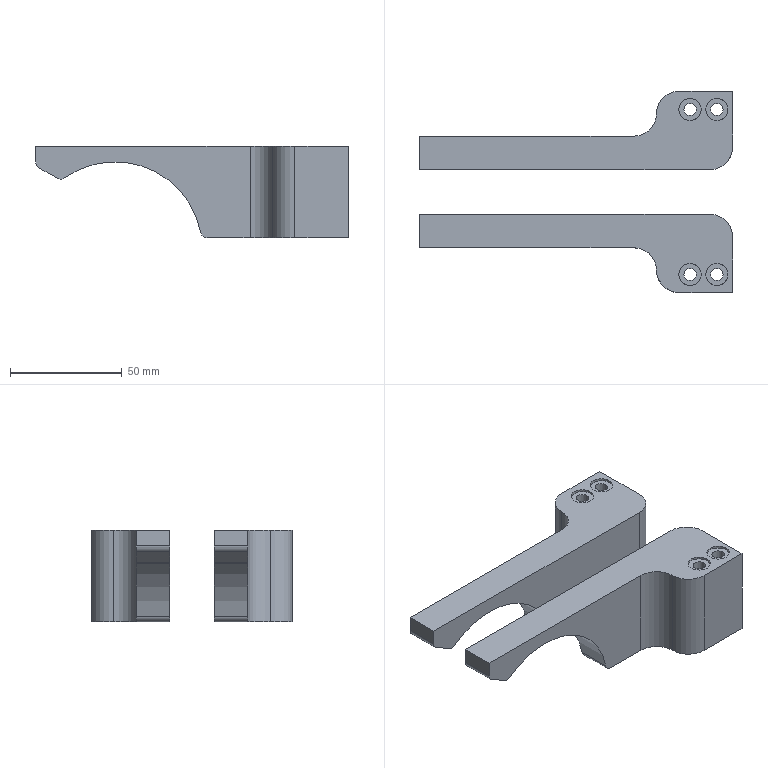NC program | NX | posted with a generic post | part box 140 x 90 x 41 mm
Lines 5312 to 6149 of 28919:
(FIXED_CONTOUR , TOOL : R4)
N10580 T08 M6
N10582 G54
N10584 G17 G0 G90 X6.198 Y-2.003 S9500 M3
N10586 G43 Z30. H8
N10588 Z4.4
N10590 G94 G1 Z0.371 F3000.
N10592 X6.29 Y-2.096 Z0.209
N10594 X6.41 Y-2.215 Z0.086
N10596 X6.548 Y-2.353 Z0.011
N10598 X6.695 Y-2.5 Z-0.011
N10600 X6.831 Y-2.637 Z-0.006
N10602 Y-2.773 Z-0.004
N10604 X6.558 Y-2.5 Z-0.014
N10606 X6.421 Z-0.017
N10608 X6.831 Y-2.91 Z-0.004
N10610 Y-3.046
N10612 X6.589 Y-2.804 Z-0.009
N10614 X6.427 Y-2.642 Z-0.015
N10616 X6.285 Y-2.5 Z-0.028
N10618 X6.148 Z-0.039
N10620 X6.427 Y-2.779 Z-0.013
N10622 X6.831 Y-3.183 Z-0.004
N10624 Y-3.318
N10626 X6.427 Y-2.914 Z-0.013
N10628 X6.145 Y-2.632 Z-0.037
N10630 X6.013 Y-2.5 Z-0.055
N10632 X5.877 Z-0.071
N10634 X6.181 Y-2.804 Z-0.032
N10636 X6.427 Y-3.05 Z-0.013
N10638 X6.831 Y-3.454 Z-0.004
N10640 Y-3.591
N10642 X6.427 Y-3.187 Z-0.013
N10644 X6.145 Y-2.905 Z-0.035
N10646 X5.863 Y-2.623 Z-0.07
N10648 X5.74 Y-2.5 Z-0.092
N10650 X5.605 Z-0.115
N10652 X5.863 Y-2.759 Z-0.068
N10654 X6.145 Y-3.041 Z-0.035
N10656 X6.427 Y-3.322 Z-0.013
N10658 X6.831 Y-3.726 Z-0.004
N10660 Y-3.86
N10662 X6.427 Y-3.456 Z-0.013
N10664 X6.145 Y-3.174 Z-0.035
N10666 X5.863 Y-2.892 Z-0.068
N10668 X5.582 Y-2.611 Z-0.117
N10670 X5.471 Y-2.5 Z-0.144
N10672 X5.336 Z-0.174
N10674 X5.582 Y-2.746 Z-0.115
N10676 X5.863 Y-3.027 Z-0.068
N10678 X6.145 Y-3.309 Z-0.035
N10680 X6.427 Y-3.591 Z-0.013
N10682 X6.831 Y-3.995 Z-0.004
N10684 Y-4.13
N10686 X6.427 Y-3.726 Z-0.013
N10688 X6.145 Y-3.445 Z-0.035
N10690 X5.863 Y-3.163 Z-0.068
N10692 X5.582 Y-2.881 Z-0.114
N10694 X5.201 Y-2.5 Z-0.206
N10696 X5.065 Z-0.238
N10698 X5.369 Y-2.804 Z-0.163
N10700 X5.582 Y-3.017 Z-0.114
N10702 X5.863 Y-3.298 Z-0.068
N10704 X6.145 Y-3.58 Z-0.035
N10706 X6.427 Y-3.862 Z-0.013
N10708 X6.831 Y-4.266 Z-0.004
N10710 Y-4.401
N10712 X6.427 Y-3.997 Z-0.013
N10714 X6.145 Y-3.715 Z-0.035
N10716 X5.863 Y-3.433 Z-0.068
N10718 X5.582 Y-3.152 Z-0.114
N10720 X5.234 Y-2.804 Z-0.194
N10722 X5.018 Y-2.588 Z-0.247
N10724 X4.93 Y-2.5 Z-0.273
N10726 X4.795 Z-0.309
N10728 X5.018 Y-2.723 Z-0.245
N10730 X5.3 Y-3.004 Z-0.178
N10732 X5.582 Y-3.286 Z-0.114
N10734 X5.863 Y-3.568 Z-0.068
N10736 X6.145 Y-3.85 Z-0.035
N10738 X6.427 Y-4.131 Z-0.013
N10740 X6.831 Y-4.536 Z-0.004
N10742 Y-4.667
N10744 X6.427 Y-4.263 Z-0.013
N10746 X6.145 Y-3.982 Z-0.035
N10748 X5.863 Y-3.7 Z-0.068
N10750 X5.582 Y-3.418 Z-0.114
N10752 X5.018 Y-2.855 Z-0.244
N10754 X4.736 Y-2.573 Z-0.324
N10756 X4.664 Y-2.5 Z-0.351
N10758 X4.531 Z-0.398
N10760 X4.736 Y-2.705 Z-0.322
N10762 X5.018 Y-2.987 Z-0.244
N10764 X5.582 Y-3.551 Z-0.114
N10766 X5.863 Y-3.832 Z-0.068
N10768 X6.145 Y-4.114 Z-0.035
N10770 X6.427 Y-4.396 Z-0.013
N10772 X6.831 Y-4.8 Z-0.004
N10774 Y-4.933
N10776 X6.427 Y-4.529 Z-0.013
N10778 X6.145 Y-4.247 Z-0.035
N10780 X5.863 Y-3.966 Z-0.068
N10782 X5.582 Y-3.684 Z-0.114
N10784 X5.018 Y-3.12 Z-0.244
N10786 X4.736 Y-2.839 Z-0.321
N10788 X4.455 Y-2.557 Z-0.424
N10790 X4.398 Y-2.5 Z-0.448
N10792 X4.265 Z-0.501
N10794 X4.455 Y-2.689 Z-0.422
N10796 X4.736 Y-2.971 Z-0.321
N10798 X5.018 Y-3.253 Z-0.244
N10800 X5.582 Y-3.816 Z-0.114
N10802 X5.863 Y-4.098 Z-0.068
N10804 X6.145 Y-4.38 Z-0.035
N10806 X6.427 Y-4.662 Z-0.013
N10808 X6.831 Y-5.066 Z-0.004
N10810 Y-5.198
N10812 X6.427 Y-4.794 Z-0.013
N10814 X6.145 Y-4.512 Z-0.035
N10816 X5.863 Y-4.23 Z-0.068
N10818 X5.582 Y-3.949 Z-0.114
N10820 X5.018 Y-3.385 Z-0.244
N10822 X4.736 Y-3.103 Z-0.321
N10824 X4.437 Y-2.804 Z-0.427
N10826 X4.133 Y-2.5 Z-0.555
N10828 X4.002 Z-0.608
N10830 X4.306 Y-2.804 Z-0.48
N10832 X4.455 Y-2.953 Z-0.42
N10834 X4.736 Y-3.234 Z-0.321
N10836 X5.018 Y-3.516 Z-0.244
N10838 X5.582 Y-4.08 Z-0.114
N10840 X5.863 Y-4.361 Z-0.068
N10842 X6.145 Y-4.643 Z-0.035
N10844 X6.427 Y-4.925 Z-0.013
N10846 X6.831 Y-5.329 Z-0.004
N10848 Y-5.459
N10850 X6.427 Y-5.055 Z-0.013
N10852 X6.145 Y-4.773 Z-0.035
N10854 X5.863 Y-4.491 Z-0.068
N10856 X5.582 Y-4.209 Z-0.114
N10858 X5.018 Y-3.646 Z-0.244
N10860 X4.736 Y-3.364 Z-0.321
N10862 X4.455 Y-3.082 Z-0.42
N10864 X4.176 Y-2.804 Z-0.532
N10866 X3.891 Y-2.519 Z-0.654
N10868 X3.872 Y-2.5 Z-0.663
N10870 X3.744 Z-0.726
N10872 X3.891 Y-2.647 Z-0.652
N10874 X4.173 Y-2.929 Z-0.534
N10876 X4.455 Y-3.21 Z-0.42
N10878 X4.736 Y-3.492 Z-0.321
N10880 X5.018 Y-3.774 Z-0.244
N10882 X5.582 Y-4.337 Z-0.114
N10884 X5.863 Y-4.619 Z-0.068
N10886 X6.145 Y-4.901 Z-0.035
N10888 X6.427 Y-5.183 Z-0.013
N10890 X6.831 Y-5.587 Z-0.004
N10892 Y-5.717
N10894 X6.427 Y-5.313 Z-0.013
N10896 X6.145 Y-5.031 Z-0.035
N10898 X5.863 Y-4.749 Z-0.068
N10900 X5.582 Y-4.468 Z-0.114
N10902 X5.02 Y-3.907 Z-0.244
N10904 X4.736 Y-3.622 Z-0.321
N10906 X4.455 Y-3.341 Z-0.42
N10908 X3.891 Y-2.777 Z-0.65
N10910 X3.614 Y-2.5 Z-0.785
N10912 X3.487 Z-0.858
N10914 X3.609 Y-2.623 Z-0.787
N10916 X3.891 Y-2.904 Z-0.649
N10918 X4.455 Y-3.468 Z-0.42
N10920 X4.736 Y-3.75 Z-0.321
N10922 X5.018 Y-4.031 Z-0.244
N10924 X5.582 Y-4.595 Z-0.114
N10926 X5.863 Y-4.877 Z-0.068
N10928 X6.145 Y-5.158 Z-0.035
N10930 X6.427 Y-5.44 Z-0.013
N10932 X6.831 Y-5.844 Z-0.004
N10934 Y-5.968
N10936 X6.427 Y-5.563 Z-0.013
N10938 X6.145 Y-5.282 Z-0.035
N10940 X5.863 Y-5. Z-0.068
N10942 X5.582 Y-4.718 Z-0.114
N10944 X5.018 Y-4.155 Z-0.244
N10946 X4.736 Y-3.873 Z-0.321
N10948 X4.455 Y-3.591 Z-0.42
N10950 X3.891 Y-3.028 Z-0.649
N10952 X3.609 Y-2.746 Z-0.787
N10954 X3.363 Y-2.5 Z-0.93
N10956 X3.237 Z-1.004
N10958 X3.327 Y-2.59 Z-0.95
N10960 X3.609 Y-2.872 Z-0.787
N10962 X3.891 Y-3.154 Z-0.649
N10964 X4.455 Y-3.717 Z-0.42
N10966 X4.736 Y-3.999 Z-0.321
N10968 X5.018 Y-4.281 Z-0.244
N10970 X5.582 Y-4.844 Z-0.114
N10972 X5.863 Y-5.126 Z-0.068
N10974 X6.145 Y-5.408 Z-0.035
N10976 X6.427 Y-5.69 Z-0.013
N10978 X6.831 Y-6.094 Z-0.004
N10980 Y-6.221
N10982 X6.427 Y-5.817 Z-0.013
N10984 X6.145 Y-5.535 Z-0.035
N10986 X5.863 Y-5.253 Z-0.068
N10988 X5.582 Y-4.971 Z-0.114
N10990 X5.018 Y-4.408 Z-0.244
N10992 X4.736 Y-4.126 Z-0.321
N10994 X4.455 Y-3.844 Z-0.42
N10996 X3.891 Y-3.281 Z-0.649
N10998 X3.609 Y-2.999 Z-0.787
N11000 X3.327 Y-2.717 Z-0.95
N11002 X3.11 Y-2.5 Z-1.08
N11004 X3.046 Z-1.118
N11006 X2.985 Z-1.16
N11008 X3.046 Y-2.561 Z-1.117
N11010 X3.327 Y-2.843 Z-0.95
N11012 X3.609 Y-3.125 Z-0.787
N11014 X3.891 Y-3.407 Z-0.649
N11016 X4.455 Y-3.97 Z-0.42
N11018 X4.736 Y-4.252 Z-0.321
N11020 X5.018 Y-4.534 Z-0.244
N11022 X5.582 Y-5.097 Z-0.114
N11024 X5.863 Y-5.379 Z-0.068
N11026 X6.145 Y-5.661 Z-0.035
N11028 X6.427 Y-5.942 Z-0.013
N11030 X6.831 Y-6.347 Z-0.004
N11032 Y-6.469
N11034 X6.427 Y-6.065 Z-0.013
N11036 X6.145 Y-5.783 Z-0.035
N11038 X5.863 Y-5.501 Z-0.068
N11040 X5.582 Y-5.219 Z-0.114
N11042 X5.018 Y-4.656 Z-0.244
N11044 X4.736 Y-4.374 Z-0.321
N11046 X4.455 Y-4.092 Z-0.42
N11048 X3.891 Y-3.529 Z-0.649
N11050 X3.609 Y-3.247 Z-0.787
N11052 X3.327 Y-2.965 Z-0.95
N11054 X3.046 Y-2.683 Z-1.117
N11056 X2.967 Y-2.605 Z-1.169
N11058 X2.862 Y-2.5 Z-1.243
N11060 X2.764 Z-1.308
N11062 X2.74 Z-1.327
N11064 X2.764 Y-2.524 Z-1.308
N11066 X2.858 Y-2.619 Z-1.244
N11068 X2.905 Y-2.665 Z-1.21
N11070 X3.046 Y-2.806 Z-1.117
N11072 X3.327 Y-3.088 Z-0.95
N11074 X3.609 Y-3.369 Z-0.787
N11076 X3.891 Y-3.651 Z-0.649
N11078 X4.455 Y-4.215 Z-0.42
N11080 X4.736 Y-4.496 Z-0.321
N11082 X5.018 Y-4.778 Z-0.244
N11084 X5.582 Y-5.342 Z-0.114
N11086 X5.863 Y-5.624 Z-0.068
N11088 X6.145 Y-5.905 Z-0.035
N11090 X6.427 Y-6.187 Z-0.013
N11092 X6.831 Y-6.591 Z-0.004
N11094 Y-6.711
N11096 X6.427 Y-6.307 Z-0.013
N11098 X6.145 Y-6.025 Z-0.035
N11100 X5.863 Y-5.743 Z-0.068
N11102 X5.582 Y-5.461 Z-0.114
N11104 X5.018 Y-4.898 Z-0.244
N11106 X4.736 Y-4.616 Z-0.321
N11108 X4.455 Y-4.334 Z-0.42
N11110 X3.891 Y-3.771 Z-0.649
N11112 X3.609 Y-3.489 Z-0.787
N11114 X3.327 Y-3.207 Z-0.95
N11116 X3.046 Y-2.926 Z-1.117
N11118 X2.845 Y-2.725 Z-1.25
N11120 X2.764 Y-2.644 Z-1.306
N11122 X2.62 Y-2.5 Z-1.422
N11124 X2.502 Z-1.512
N11126 X2.764 Y-2.762 Z-1.304
N11128 X3.046 Y-3.044 Z-1.117
N11130 X3.327 Y-3.325 Z-0.95
N11132 X3.609 Y-3.607 Z-0.787
N11134 X3.891 Y-3.889 Z-0.649
N11136 X4.455 Y-4.452 Z-0.42
N11138 X4.736 Y-4.734 Z-0.321
N11140 X5.02 Y-5.018 Z-0.244
N11142 X5.582 Y-5.58 Z-0.114
N11144 X5.863 Y-5.861 Z-0.068
N11146 X6.145 Y-6.143 Z-0.035
N11148 X6.427 Y-6.425 Z-0.013
N11150 X6.831 Y-6.829 Z-0.004
N11152 Y-6.943
N11154 X6.427 Y-6.539 Z-0.013
N11156 X6.145 Y-6.257 Z-0.035
N11158 X5.863 Y-5.975 Z-0.068
N11160 X5.582 Y-5.693 Z-0.114
N11162 X5.018 Y-5.13 Z-0.244
N11164 X4.736 Y-4.848 Z-0.321
N11166 X4.455 Y-4.566 Z-0.42
N11168 X3.891 Y-4.003 Z-0.649
N11170 X3.609 Y-3.721 Z-0.787
N11172 X3.327 Y-3.439 Z-0.95
N11174 X3.046 Y-3.157 Z-1.117
N11176 X2.764 Y-2.876 Z-1.303
N11178 X2.451 Y-2.562 Z-1.551
N11180 X2.388 Y-2.5 Z-1.604
N11182 X2.27 Z-1.701
N11184 X2.482 Y-2.712 Z-1.525
N11186 X2.764 Y-2.994 Z-1.303
N11188 X3.046 Y-3.276 Z-1.117
N11190 X3.327 Y-3.558 Z-0.95
N11192 X3.609 Y-3.839 Z-0.787
N11194 X3.891 Y-4.121 Z-0.649
N11196 X4.455 Y-4.685 Z-0.42
N11198 X4.736 Y-4.967 Z-0.321
N11200 X5.018 Y-5.248 Z-0.244
N11202 X5.582 Y-5.812 Z-0.114
N11204 X5.863 Y-6.094 Z-0.068
N11206 X6.145 Y-6.375 Z-0.035
N11208 X6.427 Y-6.657 Z-0.013
N11210 X6.831 Y-7.061 Z-0.004
N11212 Y-7.18
N11214 X6.427 Y-6.776 Z-0.013
N11216 X6.145 Y-6.495 Z-0.035
N11218 X5.863 Y-6.213 Z-0.068
N11220 X5.582 Y-5.931 Z-0.114
N11222 X5.018 Y-5.367 Z-0.244
N11224 X4.736 Y-5.086 Z-0.321
N11226 X4.455 Y-4.804 Z-0.42
N11228 X3.891 Y-4.24 Z-0.649
N11230 X3.609 Y-3.959 Z-0.787
N11232 X3.327 Y-3.677 Z-0.95
N11234 X3.046 Y-3.395 Z-1.117
N11236 X2.764 Y-3.113 Z-1.303
N11238 X2.482 Y-2.832 Z-1.525
N11240 X2.189 Y-2.539 Z-1.766
N11242 X2.151 Y-2.5 Z-1.803
N11244 X2.032 Z-1.907
N11246 X2.06 Y-2.528 Z-1.879
N11248 X2.2 Y-2.669 Z-1.757
N11250 X2.482 Y-2.951 Z-1.525
N11252 X2.764 Y-3.232 Z-1.303
N11254 X3.046 Y-3.514 Z-1.117
N11256 X3.327 Y-3.796 Z-0.95
N11258 X3.609 Y-4.078 Z-0.787
N11260 X3.891 Y-4.359 Z-0.649
N11262 X4.455 Y-4.923 Z-0.42
N11264 X4.736 Y-5.205 Z-0.321
N11266 X5.018 Y-5.486 Z-0.244
N11268 X5.582 Y-6.05 Z-0.114
N11270 X5.863 Y-6.332 Z-0.068
N11272 X6.145 Y-6.614 Z-0.035
N11274 X6.427 Y-6.895 Z-0.013
N11276 X6.831 Y-7.299 Z-0.004
N11278 Y-7.413
N11280 X6.427 Y-7.009 Z-0.013
N11282 X6.145 Y-6.728 Z-0.035
N11284 X5.863 Y-6.446 Z-0.068
N11286 X5.582 Y-6.164 Z-0.114
N11288 X5.018 Y-5.6 Z-0.244
N11290 X4.736 Y-5.319 Z-0.321
N11292 X4.455 Y-5.037 Z-0.42
N11294 X3.891 Y-4.473 Z-0.649
N11296 X3.609 Y-4.192 Z-0.787
N11298 X3.329 Y-3.911 Z-0.949
N11300 X3.046 Y-3.628 Z-1.117
N11302 X2.764 Y-3.346 Z-1.303
N11304 X2.482 Y-3.065 Z-1.525
N11306 X2.178 Y-2.761 Z-1.776
N11308 X1.979 Y-2.561 Z-1.955
N11310 X1.917 Y-2.5 Z-2.016
N11312 X1.81 Z-2.132
N11314 X1.919 Y-2.608 Z-2.014
N11316 X1.985 Y-2.674 Z-1.951
N11318 X2.2 Y-2.89 Z-1.757
N11320 X2.482 Y-3.172 Z-1.525
N11322 X2.764 Y-3.453 Z-1.303
N11324 X3.046 Y-3.735 Z-1.117
N11326 X3.327 Y-4.017 Z-0.95
N11328 X3.609 Y-4.299 Z-0.787
N11330 X3.891 Y-4.581 Z-0.649
N11332 X4.455 Y-5.144 Z-0.42
N11334 X4.736 Y-5.426 Z-0.321
N11336 X5.018 Y-5.708 Z-0.244
N11338 X5.582 Y-6.271 Z-0.114
N11340 X5.863 Y-6.553 Z-0.068
N11342 X6.145 Y-6.835 Z-0.035
N11344 X6.427 Y-7.116 Z-0.013
N11346 X6.831 Y-7.521 Z-0.004
N11348 Y-7.629
N11350 X6.427 Y-7.225 Z-0.013
N11352 X6.145 Y-6.943 Z-0.035
N11354 X5.863 Y-6.661 Z-0.068
N11356 X5.582 Y-6.379 Z-0.114
N11358 X5.018 Y-5.816 Z-0.244
N11360 X4.736 Y-5.534 Z-0.321
N11362 X4.455 Y-5.252 Z-0.42
N11364 X3.891 Y-4.689 Z-0.649
N11366 X3.609 Y-4.407 Z-0.787
N11368 X3.327 Y-4.125 Z-0.95
N11370 X3.046 Y-3.844 Z-1.117
N11372 X2.764 Y-3.562 Z-1.303
N11374 X2.482 Y-3.28 Z-1.525
N11376 X2.2 Y-2.998 Z-1.757
N11378 X1.919 Y-2.716 Z-2.014
N11380 X1.702 Y-2.5 Z-2.25
N11382 X1.593 Z-2.37
N11384 X1.637 Y-2.544 Z-2.32
N11386 X1.919 Y-2.825 Z-2.014
N11388 X2.2 Y-3.107 Z-1.757
N11390 X2.482 Y-3.389 Z-1.525
N11392 X2.764 Y-3.671 Z-1.303
N11394 X3.046 Y-3.952 Z-1.117
N11396 X3.327 Y-4.234 Z-0.95
N11398 X3.609 Y-4.516 Z-0.787
N11400 X3.891 Y-4.798 Z-0.649
N11402 X4.455 Y-5.361 Z-0.42
N11404 X4.736 Y-5.643 Z-0.321
N11406 X5.018 Y-5.925 Z-0.244
N11408 X5.582 Y-6.488 Z-0.114
N11410 X5.863 Y-6.77 Z-0.068
N11412 X6.145 Y-7.052 Z-0.035
N11414 X6.427 Y-7.334 Z-0.013
N11416 X6.831 Y-7.738 Z-0.004
N11418 Y-7.846
N11420 X6.427 Y-7.442 Z-0.013
N11422 X6.145 Y-7.16 Z-0.035
N11424 X5.863 Y-6.879 Z-0.068
N11426 X5.582 Y-6.597 Z-0.114
N11428 X5.018 Y-6.033 Z-0.244
N11430 X4.736 Y-5.751 Z-0.321
N11432 X4.455 Y-5.47 Z-0.42
N11434 X3.891 Y-4.906 Z-0.649
N11436 X3.609 Y-4.624 Z-0.787
N11438 X3.327 Y-4.343 Z-0.95
N11440 X3.046 Y-4.061 Z-1.117
N11442 X2.764 Y-3.779 Z-1.303
N11444 X2.482 Y-3.497 Z-1.525
N11446 X2.2 Y-3.216 Z-1.757
N11448 X1.919 Y-2.934 Z-2.014
N11450 X1.637 Y-2.652 Z-2.32
N11452 X1.485 Y-2.5 Z-2.492
N11454 X1.378 Z-2.614
N11456 X1.418 Y-2.54 Z-2.566
N11458 X1.637 Y-2.759 Z-2.32
N11460 X1.919 Y-3.04 Z-2.014
N11462 X2.2 Y-3.322 Z-1.757
N11464 X2.482 Y-3.604 Z-1.525
N11466 X2.764 Y-3.886 Z-1.303
N11468 X3.046 Y-4.167 Z-1.117
N11470 X3.333 Y-4.454 Z-0.946
N11472 X3.609 Y-4.731 Z-0.787
N11474 X3.891 Y-5.013 Z-0.649
N11476 X4.455 Y-5.576 Z-0.42
N11478 X4.736 Y-5.858 Z-0.321
N11480 X5.018 Y-6.14 Z-0.244
N11482 X5.582 Y-6.703 Z-0.114
N11484 X5.863 Y-6.985 Z-0.068
N11486 X6.145 Y-7.267 Z-0.035
N11488 X6.427 Y-7.549 Z-0.013
N11490 X6.831 Y-7.953 Z-0.004
N11492 Y-8.048
N11494 X6.427 Y-7.644 Z-0.013
N11496 X6.145 Y-7.362 Z-0.035
N11498 X5.863 Y-7.081 Z-0.068
N11500 X5.582 Y-6.799 Z-0.114
N11502 X5.018 Y-6.235 Z-0.244
N11504 X4.736 Y-5.954 Z-0.321
N11506 X4.455 Y-5.672 Z-0.42
N11508 X3.891 Y-5.108 Z-0.649
N11510 X3.609 Y-4.827 Z-0.787
N11512 X3.327 Y-4.545 Z-0.95
N11514 X3.046 Y-4.263 Z-1.117
N11516 X2.764 Y-3.981 Z-1.303
N11518 X2.482 Y-3.699 Z-1.525
N11520 X2.2 Y-3.418 Z-1.757
N11522 X1.919 Y-3.136 Z-2.014
N11524 X1.637 Y-2.854 Z-2.32
N11526 X1.4 Y-2.617 Z-2.588
N11528 X1.333 Y-2.551 Z-2.669
N11530 X1.283 Y-2.5 Z-2.742
N11532 X1.214 Z-2.83
N11534 X1.181 Z-2.879
N11536 X1.214 Y-2.533 Z-2.83
N11538 X1.269 Y-2.588 Z-2.757
N11540 X1.301 Y-2.62 Z-2.711
N11542 X1.355 Y-2.674 Z-2.641
N11544 X1.637 Y-2.956 Z-2.32
N11546 X1.919 Y-3.237 Z-2.014
N11548 X2.2 Y-3.519 Z-1.757
N11550 X2.482 Y-3.801 Z-1.525
N11552 X2.764 Y-4.083 Z-1.303
N11554 X3.046 Y-4.364 Z-1.117
N11556 X3.327 Y-4.646 Z-0.95
N11558 X3.609 Y-4.928 Z-0.787
N11560 X3.891 Y-5.21 Z-0.649
N11562 X4.455 Y-5.773 Z-0.42
N11564 X4.736 Y-6.055 Z-0.321
N11566 X5.018 Y-6.337 Z-0.244
N11568 X5.582 Y-6.9 Z-0.114
N11570 X5.863 Y-7.182 Z-0.068
N11572 X6.145 Y-7.464 Z-0.035
N11574 X6.427 Y-7.746 Z-0.013
N11576 X6.831 Y-8.15 Z-0.004
N11578 Y-8.251
N11580 X6.427 Y-7.847 Z-0.013
N11582 X6.145 Y-7.565 Z-0.035
N11584 X5.863 Y-7.283 Z-0.068
N11586 X5.582 Y-7.001 Z-0.114
N11588 X5.018 Y-6.438 Z-0.244
N11590 X4.736 Y-6.156 Z-0.321
N11592 X4.455 Y-5.874 Z-0.42
N11594 X3.891 Y-5.311 Z-0.649
N11596 X3.609 Y-5.029 Z-0.787
N11598 X3.327 Y-4.747 Z-0.95
N11600 X3.046 Y-4.466 Z-1.117
N11602 X2.764 Y-4.184 Z-1.303
N11604 X2.482 Y-3.902 Z-1.525
N11606 X2.2 Y-3.62 Z-1.757
N11608 X1.919 Y-3.338 Z-2.014
N11610 X1.637 Y-3.057 Z-2.32
N11612 X1.355 Y-2.775 Z-2.641
N11614 X1.269 Y-2.688 Z-2.753
N11616 X1.214 Y-2.634 Z-2.827
N11618 X1.08 Y-2.5 Z-3.027
N11620 X0.982 Z-3.177
N11622 X1.116 Y-2.635 Z-2.97
N11624 X1.214 Y-2.732 Z-2.825
N11626 X1.355 Y-2.873 Z-2.641
N11628 X1.637 Y-3.155 Z-2.32
N11630 X1.919 Y-3.437 Z-2.014
N11632 X2.2 Y-3.719 Z-1.757
N11634 X2.482 Y-4. Z-1.525
N11636 X2.764 Y-4.282 Z-1.303
N11638 X3.046 Y-4.564 Z-1.117
N11640 X3.327 Y-4.846 Z-0.95
N11642 X3.609 Y-5.127 Z-0.787
N11644 X3.891 Y-5.409 Z-0.649
N11646 X4.455 Y-5.973 Z-0.42
N11648 X4.736 Y-6.255 Z-0.321
N11650 X5.018 Y-6.536 Z-0.244
N11652 X5.582 Y-7.1 Z-0.114
N11654 X5.863 Y-7.382 Z-0.068
N11656 X6.145 Y-7.663 Z-0.035
N11658 X6.427 Y-7.945 Z-0.013
N11660 X6.831 Y-8.349 Z-0.004
N11662 Y-8.445
N11664 X6.427 Y-8.041 Z-0.013
N11666 X6.145 Y-7.759 Z-0.035
N11668 X5.863 Y-7.477 Z-0.068
N11670 X5.582 Y-7.196 Z-0.114
N11672 X5.018 Y-6.632 Z-0.244
N11674 X4.736 Y-6.35 Z-0.321
N11676 X4.455 Y-6.068 Z-0.42
N11678 X3.891 Y-5.505 Z-0.649
N11680 X3.609 Y-5.223 Z-0.787
N11682 X3.327 Y-4.941 Z-0.95
N11684 X3.046 Y-4.66 Z-1.117
N11686 X2.764 Y-4.378 Z-1.303
N11688 X2.482 Y-4.096 Z-1.525
N11690 X2.2 Y-3.814 Z-1.757
N11692 X1.919 Y-3.532 Z-2.014
N11694 X1.637 Y-3.251 Z-2.32
N11696 X1.355 Y-2.969 Z-2.641
N11698 X1.214 Y-2.828 Z-2.823
N11700 X1.073 Y-2.687 Z-3.032
N11702 X0.886 Y-2.5 Z-3.323
N11704 X0.793 Z-3.465
N11706 X1.098 Y-2.804 Z-2.994
N11708 X1.214 Y-2.921 Z-2.823
N11710 X1.355 Y-3.061 Z-2.641
N11712 X1.637 Y-3.343 Z-2.32
N11714 X1.919 Y-3.625 Z-2.014
N11716 X2.2 Y-3.907 Z-1.757
N11718 X2.482 Y-4.188 Z-1.525
N11720 X2.764 Y-4.47 Z-1.303
N11722 X3.046 Y-4.752 Z-1.117
N11724 X3.327 Y-5.034 Z-0.95
N11726 X3.609 Y-5.316 Z-0.787
N11728 X3.891 Y-5.597 Z-0.649
N11730 X4.455 Y-6.161 Z-0.42
N11732 X4.736 Y-6.443 Z-0.321
N11734 X5.018 Y-6.724 Z-0.244
N11736 X5.582 Y-7.288 Z-0.114
N11738 X5.863 Y-7.57 Z-0.068
N11740 X6.145 Y-7.852 Z-0.035
N11742 X6.427 Y-8.133 Z-0.013
N11744 X6.831 Y-8.537 Z-0.004
N11746 Y-8.623
N11748 X6.427 Y-8.219 Z-0.013
N11750 X6.145 Y-7.937 Z-0.035
N11752 X5.863 Y-7.656 Z-0.068
N11754 X5.582 Y-7.374 Z-0.114
N11756 X5.018 Y-6.81 Z-0.244
N11758 X4.736 Y-6.528 Z-0.321
N11760 X4.455 Y-6.247 Z-0.42
N11762 X3.891 Y-5.683 Z-0.649
N11764 X3.609 Y-5.401 Z-0.787
N11766 X3.327 Y-5.12 Z-0.95
N11768 X3.046 Y-4.838 Z-1.117
N11770 X2.764 Y-4.556 Z-1.303
N11772 X2.482 Y-4.274 Z-1.525
N11774 X2.2 Y-3.993 Z-1.757
N11776 X1.919 Y-3.711 Z-2.014
N11778 X1.637 Y-3.429 Z-2.32
N11780 X1.355 Y-3.147 Z-2.641
N11782 X1.214 Y-3.006 Z-2.823
N11784 X1.073 Y-2.865 Z-3.029
N11786 X0.792 Y-2.584 Z-3.466
N11788 X0.708 Y-2.5 Z-3.615
N11790 X0.651 Z-3.715
N11792 X0.627 Z-3.765
N11794 X0.654 Y-2.527 Z-3.707
N11796 X0.792 Y-2.664 Z-3.466
N11798 X1.073 Y-2.946 Z-3.029
N11800 X1.214 Y-3.087 Z-2.823
N11802 X1.355 Y-3.228 Z-2.641
N11804 X1.637 Y-3.51 Z-2.32
N11806 X1.919 Y-3.792 Z-2.014
N11808 X2.2 Y-4.073 Z-1.757
N11810 X2.482 Y-4.355 Z-1.525
N11812 X2.764 Y-4.637 Z-1.303
N11814 X3.046 Y-4.919 Z-1.117
N11816 X3.327 Y-5.2 Z-0.95
N11818 X3.609 Y-5.482 Z-0.787
N11820 X3.891 Y-5.764 Z-0.649
N11822 X4.455 Y-6.328 Z-0.42
N11824 X4.736 Y-6.609 Z-0.321
N11826 X5.018 Y-6.891 Z-0.244
N11828 X5.582 Y-7.455 Z-0.114
N11830 X5.863 Y-7.736 Z-0.068
N11832 X6.145 Y-8.018 Z-0.035
N11834 X6.427 Y-8.3 Z-0.013
N11836 X6.831 Y-8.704 Z-0.004
N11838 Y-8.781
N11840 X6.427 Y-8.377 Z-0.013
N11842 X6.145 Y-8.095 Z-0.035
N11844 X5.863 Y-7.813 Z-0.068
N11846 X5.582 Y-7.532 Z-0.114
N11848 X5.018 Y-6.968 Z-0.244
N11850 X4.736 Y-6.686 Z-0.321
N11852 X4.455 Y-6.405 Z-0.42
N11854 X3.891 Y-5.841 Z-0.649
N11856 X3.609 Y-5.559 Z-0.787
N11858 X3.327 Y-5.278 Z-0.95
N11860 X3.046 Y-4.996 Z-1.117
N11862 X2.764 Y-4.714 Z-1.303
N11864 X2.482 Y-4.432 Z-1.525
N11866 X2.2 Y-4.15 Z-1.757
N11868 X1.919 Y-3.869 Z-2.014
N11870 X1.637 Y-3.587 Z-2.32
N11872 X1.355 Y-3.305 Z-2.641
N11874 X1.214 Y-3.164 Z-2.823
N11876 X1.073 Y-3.023 Z-3.029
N11878 X0.792 Y-2.742 Z-3.466
N11880 X0.651 Y-2.601 Z-3.714
N11882 X0.55 Y-2.5 Z-3.928
N11884 X0.473 Z-4.095
N11886 X0.51 Y-2.537 Z-4.01
N11888 X0.651 Y-2.678 Z-3.714
N11890 X0.792 Y-2.819 Z-3.466
N11892 X1.073 Y-3.1 Z-3.029
N11894 X1.214 Y-3.241 Z-2.823
N11896 X1.355 Y-3.382 Z-2.641
N11898 X1.637 Y-3.664 Z-2.32
N11900 X1.919 Y-3.946 Z-2.014
N11902 X2.2 Y-4.228 Z-1.757
N11904 X2.482 Y-4.509 Z-1.525
N11906 X2.764 Y-4.791 Z-1.303
N11908 X3.046 Y-5.073 Z-1.117
N11910 X3.327 Y-5.355 Z-0.95
N11912 X3.609 Y-5.636 Z-0.787
N11914 X3.891 Y-5.918 Z-0.649
N11916 X4.455 Y-6.482 Z-0.42
N11918 X4.736 Y-6.763 Z-0.321
N11920 X5.018 Y-7.045 Z-0.244
N11922 X5.582 Y-7.609 Z-0.114
N11924 X5.863 Y-7.891 Z-0.068
N11926 X6.145 Y-8.172 Z-0.035
N11928 X6.427 Y-8.454 Z-0.013
N11930 X6.831 Y-8.858 Z-0.004
N11932 Y-8.934
N11934 X6.427 Y-8.53 Z-0.013
N11936 X6.145 Y-8.248 Z-0.035
N11938 X5.863 Y-7.966 Z-0.068
N11940 X5.582 Y-7.684 Z-0.114
N11942 X5.018 Y-7.121 Z-0.244
N11944 X4.736 Y-6.839 Z-0.321
N11946 X4.455 Y-6.557 Z-0.42
N11948 X3.891 Y-5.994 Z-0.649
N11950 X3.609 Y-5.712 Z-0.787
N11952 X3.327 Y-5.43 Z-0.95
N11954 X3.046 Y-5.148 Z-1.117
N11956 X2.764 Y-4.867 Z-1.303
N11958 X2.482 Y-4.585 Z-1.525
N11960 X2.2 Y-4.303 Z-1.757
N11962 X1.919 Y-4.021 Z-2.014
N11964 X1.637 Y-3.739 Z-2.32
N11966 X1.355 Y-3.458 Z-2.641
N11968 X1.214 Y-3.317 Z-2.823
N11970 X1.073 Y-3.176 Z-3.029
N11972 X0.792 Y-2.894 Z-3.466
N11974 X0.651 Y-2.753 Z-3.714
N11976 X0.51 Y-2.612 Z-4.01
N11978 X0.397 Y-2.5 Z-4.263
N11980 X0.369 Z-4.326
N11982 X0.328 Z-4.429
N11984 X0.369 Y-2.541 Z-4.324
N11986 X0.51 Y-2.682 Z-4.01
N11988 X0.651 Y-2.823 Z-3.714
N11990 X0.792 Y-2.964 Z-3.466
N11992 X1.073 Y-3.245 Z-3.029
N11994 X1.214 Y-3.386 Z-2.823
N11996 X1.355 Y-3.527 Z-2.641
N11998 X1.637 Y-3.809 Z-2.32
N12000 X1.919 Y-4.091 Z-2.014
N12002 X2.2 Y-4.372 Z-1.757
N12004 X2.482 Y-4.654 Z-1.525
N12006 X2.764 Y-4.936 Z-1.303
N12008 X3.046 Y-5.218 Z-1.117
N12010 X3.327 Y-5.5 Z-0.95
N12012 X3.609 Y-5.781 Z-0.787
N12014 X3.891 Y-6.063 Z-0.649
N12016 X4.455 Y-6.627 Z-0.42
N12018 X4.736 Y-6.908 Z-0.321
N12020 X5.018 Y-7.19 Z-0.244
N12022 X5.582 Y-7.754 Z-0.114
N12024 X5.863 Y-8.035 Z-0.068
N12026 X6.145 Y-8.317 Z-0.035
N12028 X6.427 Y-8.599 Z-0.013
N12030 X6.831 Y-9.003 Z-0.004
N12032 Y-9.071
N12034 X6.427 Y-8.667 Z-0.013
N12036 X6.145 Y-8.385 Z-0.035
N12038 X5.863 Y-8.104 Z-0.068
N12040 X5.582 Y-7.822 Z-0.114
N12042 X5.018 Y-7.258 Z-0.244
N12044 X4.736 Y-6.976 Z-0.321
N12046 X4.455 Y-6.695 Z-0.42
N12048 X3.891 Y-6.131 Z-0.649
N12050 X3.609 Y-5.849 Z-0.787
N12052 X3.332 Y-5.572 Z-0.947
N12054 X3.046 Y-5.286 Z-1.117
N12056 X2.764 Y-5.004 Z-1.303
N12058 X2.482 Y-4.722 Z-1.525
N12060 X2.2 Y-4.441 Z-1.757
N12062 X1.919 Y-4.159 Z-2.014
N12064 X1.637 Y-3.877 Z-2.32
N12066 X1.355 Y-3.595 Z-2.641
N12068 X1.214 Y-3.454 Z-2.823
N12070 X1.073 Y-3.313 Z-3.029
N12072 X0.792 Y-3.032 Z-3.466
N12074 X0.651 Y-2.891 Z-3.714
N12076 X0.51 Y-2.75 Z-4.01
N12078 X0.369 Y-2.609 Z-4.324
N12080 X0.26 Y-2.5 Z-4.599
N12082 X0.228 Z-4.679
N12084 X0.201 Z-4.772
N12086 X0.228 Y-2.527 Z-4.677
N12088 X0.369 Y-2.668 Z-4.324
N12090 X0.51 Y-2.809 Z-4.01
N12092 X0.651 Y-2.95 Z-3.714
N12094 X0.792 Y-3.091 Z-3.466
N12096 X1.073 Y-3.373 Z-3.029
N12098 X1.214 Y-3.514 Z-2.823
N12100 X1.355 Y-3.654 Z-2.641
N12102 X1.637 Y-3.936 Z-2.32
N12104 X1.919 Y-4.218 Z-2.014
N12106 X2.2 Y-4.5 Z-1.757
N12108 X2.482 Y-4.782 Z-1.525
N12110 X2.764 Y-5.063 Z-1.303
N12112 X3.046 Y-5.345 Z-1.117
N12114 X3.327 Y-5.627 Z-0.95
N12116 X3.609 Y-5.909 Z-0.787
N12118 X3.891 Y-6.19 Z-0.649
N12120 X4.455 Y-6.754 Z-0.42
N12122 X4.736 Y-7.036 Z-0.321
N12124 X5.018 Y-7.317 Z-0.244
N12126 X5.582 Y-7.881 Z-0.114
N12128 X5.863 Y-8.163 Z-0.068
N12130 X6.145 Y-8.445 Z-0.035
N12132 X6.427 Y-8.726 Z-0.013
N12134 X6.831 Y-9.13 Z-0.004
N12136 Y-9.184
N12138 X6.427 Y-8.78 Z-0.013
N12140 X6.145 Y-8.499 Z-0.035
N12142 X5.863 Y-8.217 Z-0.068
N12144 X5.582 Y-7.935 Z-0.114
N12146 X5.018 Y-7.371 Z-0.244
N12148 X4.736 Y-7.09 Z-0.321
N12150 X4.455 Y-6.808 Z-0.42
N12152 X3.891 Y-6.244 Z-0.649
N12154 X3.609 Y-5.963 Z-0.787
N12156 X3.327 Y-5.681 Z-0.95
N12158 X3.046 Y-5.399 Z-1.117
N12160 X2.764 Y-5.117 Z-1.303
N12162 X2.482 Y-4.836 Z-1.525
N12164 X2.2 Y-4.554 Z-1.757
N12166 X1.919 Y-4.272 Z-2.014
N12168 X1.637 Y-3.99 Z-2.32
N12170 X1.355 Y-3.708 Z-2.641
N12172 X1.214 Y-3.568 Z-2.823
N12174 X1.073 Y-3.427 Z-3.029
N12176 X0.792 Y-3.145 Z-3.466
N12178 X0.651 Y-3.004 Z-3.714
N12180 X0.51 Y-2.863 Z-4.01
N12182 X0.369 Y-2.722 Z-4.324
N12184 X0.228 Y-2.581 Z-4.677
N12186 X0.147 Y-2.5 Z-4.957
N12188 X0.091 Z-5.145
N12190 X0.228 Y-2.637 Z-4.677
N12192 X0.369 Y-2.777 Z-4.324
N12194 X0.51 Y-2.918 Z-4.01
N12196 X0.651 Y-3.059 Z-3.714
N12198 X0.792 Y-3.2 Z-3.466
N12200 X1.073 Y-3.482 Z-3.029
N12202 X1.214 Y-3.623 Z-2.823
N12204 X1.355 Y-3.764 Z-2.641
N12206 X1.637 Y-4.045 Z-2.32
N12208 X1.919 Y-4.327 Z-2.014
N12210 X2.2 Y-4.609 Z-1.757
N12212 X2.482 Y-4.891 Z-1.525
N12214 X2.764 Y-5.173 Z-1.303
N12216 X3.046 Y-5.454 Z-1.117
N12218 X3.327 Y-5.736 Z-0.95
N12220 X3.609 Y-6.018 Z-0.787
N12222 X3.891 Y-6.3 Z-0.649
N12224 X4.455 Y-6.863 Z-0.42
N12226 X4.736 Y-7.145 Z-0.321
N12228 X5.018 Y-7.427 Z-0.244
N12230 X5.582 Y-7.99 Z-0.114
N12232 X5.863 Y-8.272 Z-0.068
N12234 X6.145 Y-8.554 Z-0.035
N12236 X6.427 Y-8.836 Z-0.013
N12238 X6.831 Y-9.24 Z-0.004
N12240 Y-9.293
N12242 X6.427 Y-8.889 Z-0.013
N12244 X6.145 Y-8.607 Z-0.035
N12246 X5.863 Y-8.325 Z-0.068
N12248 X5.582 Y-8.043 Z-0.114